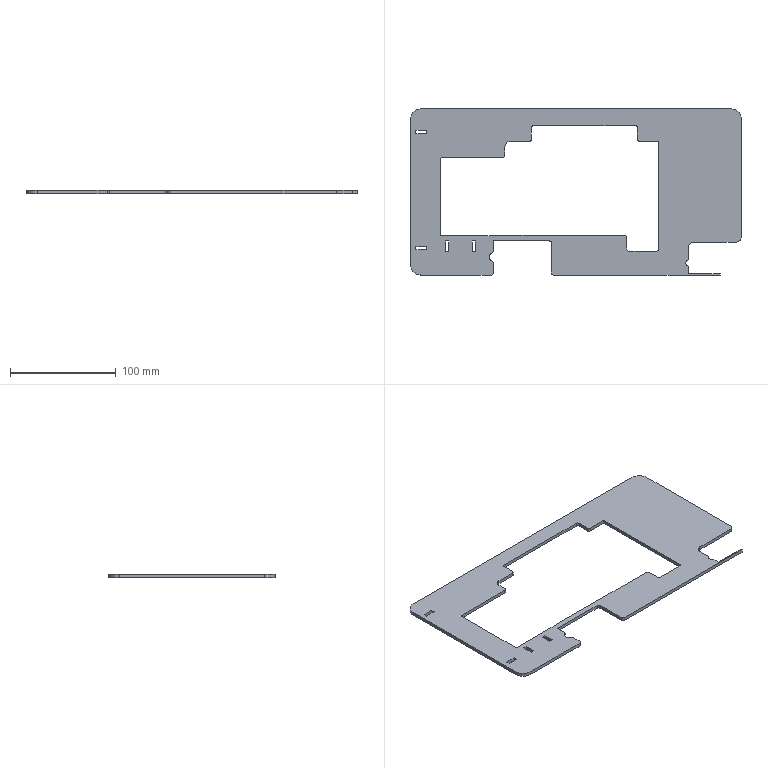Part | SolidWorks | features FlatPattern 1, SMBaseFlange 1, SheetMetal 1 | 1 solid | 72 faces | box 312.3 x 157 x 3.2 mm | volume 83817 mm3 | plane 46 | cylinder 26 | commonest cylinder face diameters 4 x16 10 x3 20 x3 5 x2 8 x2